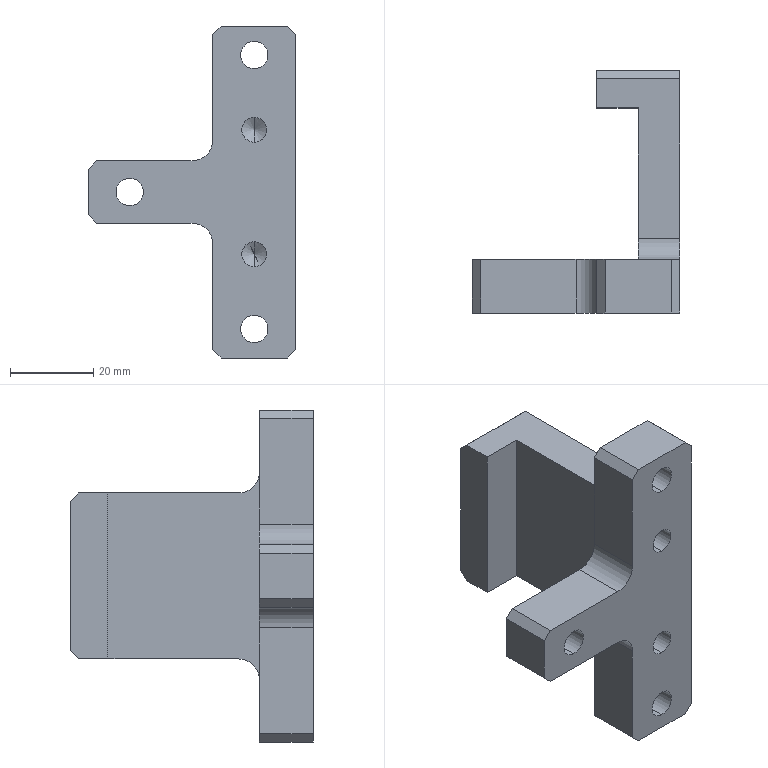Part | SolidWorks | features BaseBody 1 | 1 solid | 67 faces | box 50 x 58.5 x 80 mm | volume 45247 mm3 | cylinder 28 | plane 27 | cone 12 | commonest cylinder face diameters 2.5 x8 6.6 x6 11 x6 6 x4 10 x4